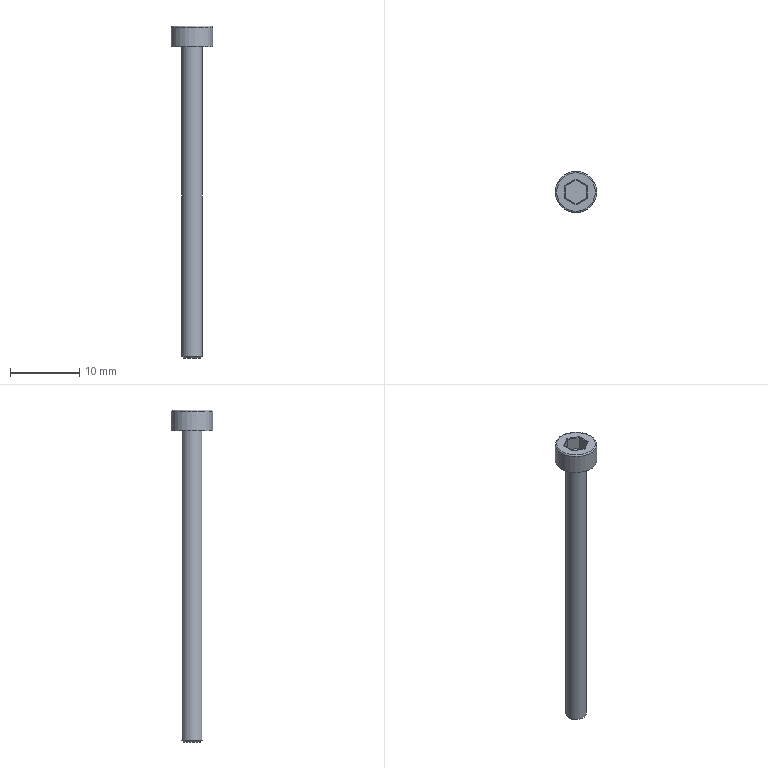Part | STEP file | 200 mesh_id626_x | 1 solid | 20 faces | box 6 x 6 x 48 mm | volume 386.861 mm3 | plane 10 | cylinder 8 | torus 1 | cone 1 | commonest cylinder face diameters 0.2 x6 3 x1 6 x1
STEP:
#1=CARTESIAN_POINT('',(-16742.034,-4013.443,137.556));
#2=VERTEX_POINT('',#1);
#3=CARTESIAN_POINT('',(-16742.034,-4011.595,137.556));
#4=VERTEX_POINT('',#3);
#5=CARTESIAN_POINT('',(-16742.034,-4012.519,137.556));
#6=DIRECTION('',(0.,1.,0.));
#7=VECTOR('',#6,1.);
#8=LINE('',#5,#7);
#9=EDGE_CURVE('',#2,#4,#8,.T.);
#10=ORIENTED_EDGE('',*,*,#9,.T.);
#11=CARTESIAN_POINT('',(-16740.434,-4010.672,137.556));
#12=VERTEX_POINT('',#11);
#13=CARTESIAN_POINT('',(-16741.234,-4011.134,137.556));
#14=DIRECTION('',(0.866,0.5,0.));
#15=VECTOR('',#14,1.);
#16=LINE('',#13,#15);
#17=EDGE_CURVE('',#4,#12,#16,.T.);
#18=ORIENTED_EDGE('',*,*,#17,.T.);
#19=CARTESIAN_POINT('',(-16738.834,-4011.595,137.556));
#20=VERTEX_POINT('',#19);
#21=CARTESIAN_POINT('',(-16739.634,-4011.134,137.556));
#22=DIRECTION('',(0.866,-0.5,0.));
#23=VECTOR('',#22,1.);
#24=LINE('',#21,#23);
#25=EDGE_CURVE('',#12,#20,#24,.T.);
#26=ORIENTED_EDGE('',*,*,#25,.T.);
#27=CARTESIAN_POINT('',(-16738.834,-4013.443,137.556));
#28=VERTEX_POINT('',#27);
#29=CARTESIAN_POINT('',(-16738.834,-4012.519,137.556));
#30=DIRECTION('',(0.,-1.,0.));
#31=VECTOR('',#30,1.);
#32=LINE('',#29,#31);
#33=EDGE_CURVE('',#20,#28,#32,.T.);
#34=ORIENTED_EDGE('',*,*,#33,.T.);
#35=CARTESIAN_POINT('',(-16740.434,-4014.367,137.556));
#36=VERTEX_POINT('',#35);
#37=CARTESIAN_POINT('',(-16739.634,-4013.905,137.556));
#38=DIRECTION('',(-0.866,-0.5,0.));
#39=VECTOR('',#38,1.);
#40=LINE('',#37,#39);
#41=EDGE_CURVE('',#28,#36,#40,.T.);
#42=ORIENTED_EDGE('',*,*,#41,.T.);
#43=CARTESIAN_POINT('',(-16741.234,-4013.905,137.556));
#44=DIRECTION('',(-0.866,0.5,0.));
#45=VECTOR('',#44,1.);
#46=LINE('',#43,#45);
#47=EDGE_CURVE('',#36,#2,#46,.T.);
#48=ORIENTED_EDGE('',*,*,#47,.T.);
#49=EDGE_LOOP('',(#10,#18,#26,#34,#42,#48));
#50=FACE_BOUND('',#49,.T.);
#51=CARTESIAN_POINT('',(-16737.634,-4012.519,137.556));
#52=VERTEX_POINT('',#51);
#53=CARTESIAN_POINT('',(-16740.434,-4012.519,137.556));
#54=DIRECTION('',(0.,0.,1.));
#55=DIRECTION('',(1.,0.,0.));
#56=AXIS2_PLACEMENT_3D('',#53,#54,#55);
#57=CIRCLE('',#56,2.8);
#58=EDGE_CURVE('',#52,#52,#57,.T.);
#59=ORIENTED_EDGE('',*,*,#58,.T.);
#60=EDGE_LOOP('',(#59));
#61=FACE_BOUND('',#60,.T.);
#62=CARTESIAN_POINT('',(-16740.434,-4012.519,137.556));
#63=DIRECTION('',(0.,0.,1.));
#64=DIRECTION('',(1.,0.,0.));
#65=AXIS2_PLACEMENT_3D('',#62,#63,#64);
#66=PLANE('',#65);
#67=ADVANCED_FACE('',(#50,#61),#66,.T.);
#68=CARTESIAN_POINT('',(-16738.934,-4012.519,134.556));
#69=VERTEX_POINT('',#68);
#70=CARTESIAN_POINT('',(-16740.434,-4012.519,134.556));
#71=DIRECTION('',(0.,0.,-1.));
#72=DIRECTION('',(1.,0.,0.));
#73=AXIS2_PLACEMENT_3D('',#70,#71,#72);
#74=CIRCLE('',#73,1.5);
#75=EDGE_CURVE('',#69,#69,#74,.T.);
#76=ORIENTED_EDGE('',*,*,#75,.F.);
#77=EDGE_LOOP('',(#76));
#78=FACE_BOUND('',#77,.T.);
#79=CARTESIAN_POINT('',(-16737.434,-4012.519,134.556));
#80=VERTEX_POINT('',#79);
#81=CARTESIAN_POINT('',(-16740.434,-4012.519,134.556));
#82=DIRECTION('',(0.,0.,1.));
#83=DIRECTION('',(1.,0.,0.));
#84=AXIS2_PLACEMENT_3D('',#81,#82,#83);
#85=CIRCLE('',#84,3.);
#86=EDGE_CURVE('',#80,#80,#85,.T.);
#87=ORIENTED_EDGE('',*,*,#86,.F.);
#88=EDGE_LOOP('',(#87));
#89=FACE_BOUND('',#88,.T.);
#90=CARTESIAN_POINT('',(-16740.434,-4012.519,134.556));
#91=DIRECTION('',(0.,0.,-1.));
#92=DIRECTION('',(-1.,0.,0.));
#93=AXIS2_PLACEMENT_3D('',#90,#91,#92);
#94=PLANE('',#93);
#95=ADVANCED_FACE('',(#78,#89),#94,.T.);
#96=CARTESIAN_POINT('',(-16737.434,-4012.519,137.356));
#97=VERTEX_POINT('',#96);
#98=CARTESIAN_POINT('',(-16740.434,-4012.519,137.356));
#99=DIRECTION('',(0.,0.,-1.));
#100=DIRECTION('',(1.,0.,0.));
#101=AXIS2_PLACEMENT_3D('',#98,#99,#100);
#102=CIRCLE('',#101,3.);
#103=EDGE_CURVE('',#97,#97,#102,.T.);
#104=ORIENTED_EDGE('',*,*,#103,.T.);
#105=EDGE_LOOP('',(#104));
#106=FACE_BOUND('',#105,.T.);
#107=ORIENTED_EDGE('',*,*,#86,.T.);
#108=EDGE_LOOP('',(#107));
#109=FACE_BOUND('',#108,.T.);
#110=CARTESIAN_POINT('',(-16740.434,-4012.519,134.556));
#111=DIRECTION('',(0.,0.,1.));
#112=DIRECTION('',(1.,0.,0.));
#113=AXIS2_PLACEMENT_3D('',#110,#111,#112);
#114=CYLINDRICAL_SURFACE('',#113,3.);
#115=ADVANCED_FACE('',(#106,#109),#114,.T.);
#116=CARTESIAN_POINT('',(-16740.434,-4010.787,135.556));
#117=VERTEX_POINT('',#116);
#118=CARTESIAN_POINT('',(-16740.434,-4010.787,137.456));
#119=VERTEX_POINT('',#118);
#120=CARTESIAN_POINT('',(-16740.434,-4010.787,137.556));
#121=DIRECTION('',(0.,0.,1.));
#122=VECTOR('',#121,1.);
#123=LINE('',#120,#122);
#124=EDGE_CURVE('',#117,#119,#123,.T.);
#125=ORIENTED_EDGE('',*,*,#124,.T.);
#126=CARTESIAN_POINT('',(-16741.934,-4011.653,137.456));
#127=VERTEX_POINT('',#126);
#128=CARTESIAN_POINT('',(-16740.434,-4010.787,137.456));
#129=DIRECTION('',(-0.866,-0.5,0.));
#130=VECTOR('',#129,1.);
#131=LINE('',#128,#130);
#132=EDGE_CURVE('',#119,#127,#131,.T.);
#133=ORIENTED_EDGE('',*,*,#132,.T.);
#134=CARTESIAN_POINT('',(-16741.934,-4011.653,135.556));
#135=VERTEX_POINT('',#134);
#136=CARTESIAN_POINT('',(-16741.934,-4011.653,137.556));
#137=DIRECTION('',(0.,0.,1.));
#138=VECTOR('',#137,1.);
#139=LINE('',#136,#138);
#140=EDGE_CURVE('',#135,#127,#139,.T.);
#141=ORIENTED_EDGE('',*,*,#140,.F.);
#142=CARTESIAN_POINT('',(-16740.434,-4010.787,135.556));
#143=DIRECTION('',(0.866,0.5,0.));
#144=VECTOR('',#143,1.);
#145=LINE('',#142,#144);
#146=EDGE_CURVE('',#135,#117,#145,.T.);
#147=ORIENTED_EDGE('',*,*,#146,.T.);
#148=EDGE_LOOP('',(#125,#133,#141,#147));
#149=FACE_OUTER_BOUND('',#148,.T.);
#150=CARTESIAN_POINT('',(-16740.434,-4010.787,137.556));
#151=DIRECTION('',(0.5,-0.866,0.));
#152=DIRECTION('',(0.866,0.5,0.));
#153=AXIS2_PLACEMENT_3D('',#150,#151,#152);
#154=PLANE('',#153);
#155=ADVANCED_FACE('',(#149),#154,.T.);
#156=ORIENTED_EDGE('',*,*,#140,.T.);
#157=CARTESIAN_POINT('',(-16741.934,-4013.385,137.456));
#158=VERTEX_POINT('',#157);
#159=CARTESIAN_POINT('',(-16741.934,-4011.653,137.456));
#160=DIRECTION('',(0.,-1.,0.));
#161=VECTOR('',#160,1.);
#162=LINE('',#159,#161);
#163=EDGE_CURVE('',#127,#158,#162,.T.);
#164=ORIENTED_EDGE('',*,*,#163,.T.);
#165=CARTESIAN_POINT('',(-16741.934,-4013.385,135.556));
#166=VERTEX_POINT('',#165);
#167=CARTESIAN_POINT('',(-16741.934,-4013.385,137.556));
#168=DIRECTION('',(0.,0.,1.));
#169=VECTOR('',#168,1.);
#170=LINE('',#167,#169);
#171=EDGE_CURVE('',#166,#158,#170,.T.);
#172=ORIENTED_EDGE('',*,*,#171,.F.);
#173=CARTESIAN_POINT('',(-16741.934,-4011.653,135.556));
#174=DIRECTION('',(0.,1.,0.));
#175=VECTOR('',#174,1.);
#176=LINE('',#173,#175);
#177=EDGE_CURVE('',#166,#135,#176,.T.);
#178=ORIENTED_EDGE('',*,*,#177,.T.);
#179=EDGE_LOOP('',(#156,#164,#172,#178));
#180=FACE_OUTER_BOUND('',#179,.T.);
#181=CARTESIAN_POINT('',(-16741.934,-4011.653,137.556));
#182=DIRECTION('',(1.,0.,0.));
#183=DIRECTION('',(0.,0.,-1.));
#184=AXIS2_PLACEMENT_3D('',#181,#182,#183);
#185=PLANE('',#184);
#186=ADVANCED_FACE('',(#180),#185,.T.);
#187=ORIENTED_EDGE('',*,*,#171,.T.);
#188=CARTESIAN_POINT('',(-16740.434,-4014.251,137.456));
#189=VERTEX_POINT('',#188);
#190=CARTESIAN_POINT('',(-16741.934,-4013.385,137.456));
#191=DIRECTION('',(0.866,-0.5,0.));
#192=VECTOR('',#191,1.);
#193=LINE('',#190,#192);
#194=EDGE_CURVE('',#158,#189,#193,.T.);
#195=ORIENTED_EDGE('',*,*,#194,.T.);
#196=CARTESIAN_POINT('',(-16740.434,-4014.251,135.556));
#197=VERTEX_POINT('',#196);
#198=CARTESIAN_POINT('',(-16740.434,-4014.251,137.556));
#199=DIRECTION('',(0.,0.,1.));
#200=VECTOR('',#199,1.);
#201=LINE('',#198,#200);
#202=EDGE_CURVE('',#197,#189,#201,.T.);
#203=ORIENTED_EDGE('',*,*,#202,.F.);
#204=CARTESIAN_POINT('',(-16741.934,-4013.385,135.556));
#205=DIRECTION('',(-0.866,0.5,0.));
#206=VECTOR('',#205,1.);
#207=LINE('',#204,#206);
#208=EDGE_CURVE('',#197,#166,#207,.T.);
#209=ORIENTED_EDGE('',*,*,#208,.T.);
#210=EDGE_LOOP('',(#187,#195,#203,#209));
#211=FACE_OUTER_BOUND('',#210,.T.);
#212=CARTESIAN_POINT('',(-16741.934,-4013.385,137.556));
#213=DIRECTION('',(0.5,0.866,0.));
#214=DIRECTION('',(-0.866,0.5,0.));
#215=AXIS2_PLACEMENT_3D('',#212,#213,#214);
#216=PLANE('',#215);
#217=ADVANCED_FACE('',(#211),#216,.T.);
#218=ORIENTED_EDGE('',*,*,#202,.T.);
#219=CARTESIAN_POINT('',(-16738.934,-4013.385,137.456));
#220=VERTEX_POINT('',#219);
#221=CARTESIAN_POINT('',(-16740.434,-4014.251,137.456));
#222=DIRECTION('',(0.866,0.5,0.));
#223=VECTOR('',#222,1.);
#224=LINE('',#221,#223);
#225=EDGE_CURVE('',#189,#220,#224,.T.);
#226=ORIENTED_EDGE('',*,*,#225,.T.);
#227=CARTESIAN_POINT('',(-16738.934,-4013.385,135.556));
#228=VERTEX_POINT('',#227);
#229=CARTESIAN_POINT('',(-16738.934,-4013.385,137.556));
#230=DIRECTION('',(0.,0.,1.));
#231=VECTOR('',#230,1.);
#232=LINE('',#229,#231);
#233=EDGE_CURVE('',#228,#220,#232,.T.);
#234=ORIENTED_EDGE('',*,*,#233,.F.);
#235=CARTESIAN_POINT('',(-16740.434,-4014.251,135.556));
#236=DIRECTION('',(-0.866,-0.5,0.));
#237=VECTOR('',#236,1.);
#238=LINE('',#235,#237);
#239=EDGE_CURVE('',#228,#197,#238,.T.);
#240=ORIENTED_EDGE('',*,*,#239,.T.);
#241=EDGE_LOOP('',(#218,#226,#234,#240));
#242=FACE_OUTER_BOUND('',#241,.T.);
#243=CARTESIAN_POINT('',(-16740.434,-4014.251,137.556));
#244=DIRECTION('',(-0.5,0.866,0.));
#245=DIRECTION('',(-0.866,-0.5,0.));
#246=AXIS2_PLACEMENT_3D('',#243,#244,#245);
#247=PLANE('',#246);
#248=ADVANCED_FACE('',(#242),#247,.T.);
#249=ORIENTED_EDGE('',*,*,#233,.T.);
#250=CARTESIAN_POINT('',(-16738.934,-4011.653,137.456));
#251=VERTEX_POINT('',#250);
#252=CARTESIAN_POINT('',(-16738.934,-4013.385,137.456));
#253=DIRECTION('',(0.,1.,0.));
#254=VECTOR('',#253,1.);
#255=LINE('',#252,#254);
#256=EDGE_CURVE('',#220,#251,#255,.T.);
#257=ORIENTED_EDGE('',*,*,#256,.T.);
#258=CARTESIAN_POINT('',(-16738.934,-4011.653,135.556));
#259=VERTEX_POINT('',#258);
#260=CARTESIAN_POINT('',(-16738.934,-4011.653,137.556));
#261=DIRECTION('',(0.,0.,1.));
#262=VECTOR('',#261,1.);
#263=LINE('',#260,#262);
#264=EDGE_CURVE('',#259,#251,#263,.T.);
#265=ORIENTED_EDGE('',*,*,#264,.F.);
#266=CARTESIAN_POINT('',(-16738.934,-4013.385,135.556));
#267=DIRECTION('',(0.,-1.,0.));
#268=VECTOR('',#267,1.);
#269=LINE('',#266,#268);
#270=EDGE_CURVE('',#259,#228,#269,.T.);
#271=ORIENTED_EDGE('',*,*,#270,.T.);
#272=EDGE_LOOP('',(#249,#257,#265,#271));
#273=FACE_OUTER_BOUND('',#272,.T.);
#274=CARTESIAN_POINT('',(-16738.934,-4013.385,137.556));
#275=DIRECTION('',(-1.,0.,0.));
#276=DIRECTION('',(0.,0.,1.));
#277=AXIS2_PLACEMENT_3D('',#274,#275,#276);
#278=PLANE('',#277);
#279=ADVANCED_FACE('',(#273),#278,.T.);
#280=ORIENTED_EDGE('',*,*,#264,.T.);
#281=CARTESIAN_POINT('',(-16738.934,-4011.653,137.456));
#282=DIRECTION('',(-0.866,0.5,0.));
#283=VECTOR('',#282,1.);
#284=LINE('',#281,#283);
#285=EDGE_CURVE('',#251,#119,#284,.T.);
#286=ORIENTED_EDGE('',*,*,#285,.T.);
#287=ORIENTED_EDGE('',*,*,#124,.F.);
#288=CARTESIAN_POINT('',(-16738.934,-4011.653,135.556));
#289=DIRECTION('',(0.866,-0.5,0.));
#290=VECTOR('',#289,1.);
#291=LINE('',#288,#290);
#292=EDGE_CURVE('',#117,#259,#291,.T.);
#293=ORIENTED_EDGE('',*,*,#292,.T.);
#294=EDGE_LOOP('',(#280,#286,#287,#293));
#295=FACE_OUTER_BOUND('',#294,.T.);
#296=CARTESIAN_POINT('',(-16738.934,-4011.653,137.556));
#297=DIRECTION('',(-0.5,-0.866,0.));
#298=DIRECTION('',(0.866,-0.5,0.));
#299=AXIS2_PLACEMENT_3D('',#296,#297,#298);
#300=PLANE('',#299);
#301=ADVANCED_FACE('',(#295),#300,.T.);
#302=ORIENTED_EDGE('',*,*,#146,.F.);
#303=ORIENTED_EDGE('',*,*,#177,.F.);
#304=ORIENTED_EDGE('',*,*,#208,.F.);
#305=ORIENTED_EDGE('',*,*,#239,.F.);
#306=ORIENTED_EDGE('',*,*,#270,.F.);
#307=ORIENTED_EDGE('',*,*,#292,.F.);
#308=EDGE_LOOP('',(#302,#303,#304,#305,#306,#307));
#309=FACE_OUTER_BOUND('',#308,.T.);
#310=CARTESIAN_POINT('',(0.,0.,135.556));
#311=DIRECTION('',(0.,0.,1.));
#312=DIRECTION('',(1.,0.,0.));
#313=AXIS2_PLACEMENT_3D('',#310,#311,#312);
#314=PLANE('',#313);
#315=ADVANCED_FACE('',(#309),#314,.T.);
#316=CARTESIAN_POINT('',(-16741.684,-4012.519,89.556));
#317=VERTEX_POINT('',#316);
#318=CARTESIAN_POINT('',(-16740.434,-4012.519,89.556));
#319=DIRECTION('',(0.,0.,-1.));
#320=DIRECTION('',(-1.,0.,0.));
#321=AXIS2_PLACEMENT_3D('',#318,#319,#320);
#322=CIRCLE('',#321,1.25);
#323=EDGE_CURVE('',#317,#317,#322,.T.);
#324=ORIENTED_EDGE('',*,*,#323,.T.);
#325=EDGE_LOOP('',(#324));
#326=FACE_OUTER_BOUND('',#325,.T.);
#327=CARTESIAN_POINT('',(-16740.434,-4012.519,89.556));
#328=DIRECTION('',(0.,0.,-1.));
#329=DIRECTION('',(-1.,0.,0.));
#330=AXIS2_PLACEMENT_3D('',#327,#328,#329);
#331=PLANE('',#330);
#332=ADVANCED_FACE('',(#326),#331,.T.);
#333=CARTESIAN_POINT('',(-16741.934,-4012.519,89.806));
#334=VERTEX_POINT('',#333);
#335=CARTESIAN_POINT('',(-16740.434,-4012.519,89.806));
#336=DIRECTION('',(0.,0.,1.));
#337=DIRECTION('',(-1.,0.,0.));
#338=AXIS2_PLACEMENT_3D('',#335,#336,#337);
#339=CIRCLE('',#338,1.5);
#340=EDGE_CURVE('',#334,#334,#339,.T.);
#341=ORIENTED_EDGE('',*,*,#340,.T.);
#342=EDGE_LOOP('',(#341));
#343=FACE_BOUND('',#342,.T.);
#344=ORIENTED_EDGE('',*,*,#75,.T.);
#345=EDGE_LOOP('',(#344));
#346=FACE_BOUND('',#345,.T.);
#347=CARTESIAN_POINT('',(-16740.434,-4012.519,134.556));
#348=DIRECTION('',(0.,0.,-1.));
#349=DIRECTION('',(1.,0.,0.));
#350=AXIS2_PLACEMENT_3D('',#347,#348,#349);
#351=CYLINDRICAL_SURFACE('',#350,1.5);
#352=ADVANCED_FACE('',(#343,#346),#351,.T.);
#353=ORIENTED_EDGE('',*,*,#58,.F.);
#354=EDGE_LOOP('',(#353));
#355=FACE_BOUND('',#354,.T.);
#356=ORIENTED_EDGE('',*,*,#103,.F.);
#357=EDGE_LOOP('',(#356));
#358=FACE_BOUND('',#357,.T.);
#359=CARTESIAN_POINT('',(-16740.434,-4012.519,137.356));
#360=DIRECTION('',(0.,0.,1.));
#361=DIRECTION('',(1.,0.,0.));
#362=AXIS2_PLACEMENT_3D('',#359,#360,#361);
#363=TOROIDAL_SURFACE('',#362,2.8,0.2);
#364=ADVANCED_FACE('',(#355,#358),#363,.T.);
#365=CARTESIAN_POINT('',(-16740.434,-4014.367,137.456));
#366=DIRECTION('',(-1.,0.,0.));
#367=DIRECTION('',(0.,1.,0.));
#368=AXIS2_PLACEMENT_3D('',#365,#366,#367);
#369=ELLIPSE('',#368,0.1155,0.1);
#370=EDGE_CURVE('',#36,#189,#369,.T.);
#371=ORIENTED_EDGE('',*,*,#370,.F.);
#372=ORIENTED_EDGE('',*,*,#41,.F.);
#373=CARTESIAN_POINT('',(-16738.834,-4013.443,137.456));
#374=DIRECTION('',(0.5,0.866,0.));
#375=DIRECTION('',(-0.866,0.5,0.));
#376=AXIS2_PLACEMENT_3D('',#373,#374,#375);
#377=ELLIPSE('',#376,0.1155,0.1);
#378=EDGE_CURVE('',#220,#28,#377,.T.);
#379=ORIENTED_EDGE('',*,*,#378,.F.);
#380=ORIENTED_EDGE('',*,*,#225,.F.);
#381=EDGE_LOOP('',(#371,#372,#379,#380));
#382=FACE_OUTER_BOUND('',#381,.T.);
#383=CARTESIAN_POINT('',(-16740.384,-4014.338,137.456));
#384=DIRECTION('',(0.866,0.5,0.));
#385=DIRECTION('',(-0.5,0.866,0.));
#386=AXIS2_PLACEMENT_3D('',#383,#384,#385);
#387=CYLINDRICAL_SURFACE('',#386,0.1);
#388=ADVANCED_FACE('',(#382),#387,.T.);
#389=ORIENTED_EDGE('',*,*,#378,.T.);
#390=ORIENTED_EDGE('',*,*,#33,.F.);
#391=CARTESIAN_POINT('',(-16738.834,-4011.595,137.456));
#392=DIRECTION('',(-0.5,0.866,0.));
#393=DIRECTION('',(-0.866,-0.5,0.));
#394=AXIS2_PLACEMENT_3D('',#391,#392,#393);
#395=ELLIPSE('',#394,0.1155,0.1);
#396=EDGE_CURVE('',#251,#20,#395,.T.);
#397=ORIENTED_EDGE('',*,*,#396,.F.);
#398=ORIENTED_EDGE('',*,*,#256,.F.);
#399=EDGE_LOOP('',(#389,#390,#397,#398));
#400=FACE_OUTER_BOUND('',#399,.T.);
#401=CARTESIAN_POINT('',(-16738.834,-4013.385,137.456));
#402=DIRECTION('',(0.,1.,0.));
#403=DIRECTION('',(0.,0.,1.));
#404=AXIS2_PLACEMENT_3D('',#401,#402,#403);
#405=CYLINDRICAL_SURFACE('',#404,0.1);
#406=ADVANCED_FACE('',(#400),#405,.T.);
#407=ORIENTED_EDGE('',*,*,#370,.T.);
#408=ORIENTED_EDGE('',*,*,#194,.F.);
#409=CARTESIAN_POINT('',(-16742.034,-4013.443,137.456));
#410=DIRECTION('',(-0.5,0.866,0.));
#411=DIRECTION('',(0.866,0.5,0.));
#412=AXIS2_PLACEMENT_3D('',#409,#410,#411);
#413=ELLIPSE('',#412,0.1155,0.1);
#414=EDGE_CURVE('',#2,#158,#413,.T.);
#415=ORIENTED_EDGE('',*,*,#414,.F.);
#416=ORIENTED_EDGE('',*,*,#47,.F.);
#417=EDGE_LOOP('',(#407,#408,#415,#416));
#418=FACE_OUTER_BOUND('',#417,.T.);
#419=CARTESIAN_POINT('',(-16741.984,-4013.472,137.456));
#420=DIRECTION('',(0.866,-0.5,0.));
#421=DIRECTION('',(0.5,0.866,0.));
#422=AXIS2_PLACEMENT_3D('',#419,#420,#421);
#423=CYLINDRICAL_SURFACE('',#422,0.1);
#424=ADVANCED_FACE('',(#418),#423,.T.);
#425=ORIENTED_EDGE('',*,*,#396,.T.);
#426=ORIENTED_EDGE('',*,*,#25,.F.);
#427=CARTESIAN_POINT('',(-16740.434,-4010.672,137.456));
#428=DIRECTION('',(-1.,0.,0.));
#429=DIRECTION('',(0.,-1.,0.));
#430=AXIS2_PLACEMENT_3D('',#427,#428,#429);
#431=ELLIPSE('',#430,0.1155,0.1);
#432=EDGE_CURVE('',#119,#12,#431,.T.);
#433=ORIENTED_EDGE('',*,*,#432,.F.);
#434=ORIENTED_EDGE('',*,*,#285,.F.);
#435=EDGE_LOOP('',(#425,#426,#433,#434));
#436=FACE_OUTER_BOUND('',#435,.T.);
#437=CARTESIAN_POINT('',(-16738.884,-4011.567,137.456));
#438=DIRECTION('',(-0.866,0.5,0.));
#439=DIRECTION('',(-0.5,-0.866,0.));
#440=AXIS2_PLACEMENT_3D('',#437,#438,#439);
#441=CYLINDRICAL_SURFACE('',#440,0.1);
#442=ADVANCED_FACE('',(#436),#441,.T.);
#443=ORIENTED_EDGE('',*,*,#414,.T.);
#444=ORIENTED_EDGE('',*,*,#163,.F.);
#445=CARTESIAN_POINT('',(-16742.034,-4011.595,137.456));
#446=DIRECTION('',(0.5,0.866,0.));
#447=DIRECTION('',(-0.866,0.5,0.));
#448=AXIS2_PLACEMENT_3D('',#445,#446,#447);
#449=ELLIPSE('',#448,0.1155,0.1);
#450=EDGE_CURVE('',#4,#127,#449,.T.);
#451=ORIENTED_EDGE('',*,*,#450,.F.);
#452=ORIENTED_EDGE('',*,*,#9,.F.);
#453=EDGE_LOOP('',(#443,#444,#451,#452));
#454=FACE_OUTER_BOUND('',#453,.T.);
#455=CARTESIAN_POINT('',(-16742.034,-4011.653,137.456));
#456=DIRECTION('',(0.,-1.,0.));
#457=DIRECTION('',(0.,0.,-1.));
#458=AXIS2_PLACEMENT_3D('',#455,#456,#457);
#459=CYLINDRICAL_SURFACE('',#458,0.1);
#460=ADVANCED_FACE('',(#454),#459,.T.);
#461=ORIENTED_EDGE('',*,*,#432,.T.);
#462=ORIENTED_EDGE('',*,*,#17,.F.);
#463=ORIENTED_EDGE('',*,*,#450,.T.);
#464=ORIENTED_EDGE('',*,*,#132,.F.);
#465=EDGE_LOOP('',(#461,#462,#463,#464));
#466=FACE_OUTER_BOUND('',#465,.T.);
#467=CARTESIAN_POINT('',(-16740.484,-4010.701,137.456));
#468=DIRECTION('',(-0.866,-0.5,0.));
#469=DIRECTION('',(0.5,-0.866,0.));
#470=AXIS2_PLACEMENT_3D('',#467,#468,#469);
#471=CYLINDRICAL_SURFACE('',#470,0.1);
#472=ADVANCED_FACE('',(#466),#471,.T.);
#473=ORIENTED_EDGE('',*,*,#323,.F.);
#474=EDGE_LOOP('',(#473));
#475=FACE_BOUND('',#474,.T.);
#476=ORIENTED_EDGE('',*,*,#340,.F.);
#477=EDGE_LOOP('',(#476));
#478=FACE_BOUND('',#477,.T.);
#479=CARTESIAN_POINT('',(-16740.434,-4012.519,89.806));
#480=DIRECTION('',(0.,0.,1.));
#481=DIRECTION('',(1.,0.,0.));
#482=AXIS2_PLACEMENT_3D('',#479,#480,#481);
#483=CONICAL_SURFACE('',#482,1.5,45.);
#484=ADVANCED_FACE('',(#475,#478),#483,.T.);
#485=CLOSED_SHELL('',(#67,#95,#115,#155,#186,#217,#248,#279,#301,#315,#332,#352,#364,#388,#406,#424,#442,#460,#472,#484));
#486=MANIFOLD_SOLID_BREP('',#485);
#487=(LENGTH_UNIT()NAMED_UNIT(*)SI_UNIT(.MILLI.,.METRE.));
#488=UNCERTAINTY_MEASURE_WITH_UNIT(LENGTH_MEASURE(0.00002),#487,'','');
#489=(NAMED_UNIT(*)PLANE_ANGLE_UNIT()SI_UNIT($,.RADIAN.));
#490=PLANE_ANGLE_MEASURE_WITH_UNIT(PLANE_ANGLE_MEASURE(0.01745),#489);
#491=DIMENSIONAL_EXPONENTS(0.,0.,0.,0.,0.,0.,0.);
#492=(CONVERSION_BASED_UNIT('DEGREE',#490)NAMED_UNIT(#491)PLANE_ANGLE_UNIT());
#493=(NAMED_UNIT(*)SI_UNIT($,.STERADIAN.)SOLID_ANGLE_UNIT());
#494=(GEOMETRIC_REPRESENTATION_CONTEXT(3)GLOBAL_UNCERTAINTY_ASSIGNED_CONTEXT((#488))GLOBAL_UNIT_ASSIGNED_CONTEXT((#487,#492,#493))REPRESENTATION_CONTEXT('',''));
#495=ADVANCED_BREP_SHAPE_REPRESENTATION('',(#486),#494);